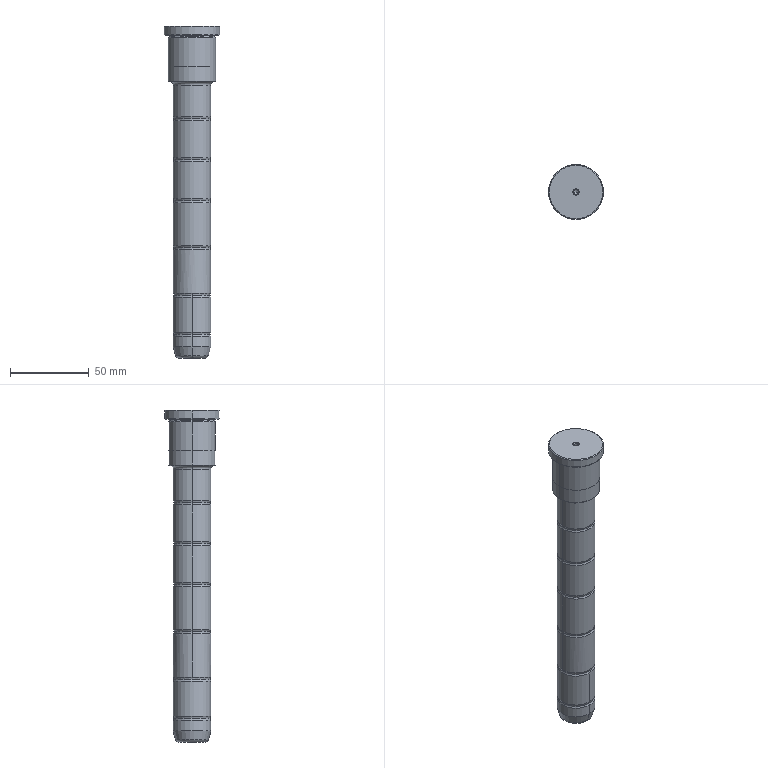Part | STEP file | Coluna inferior | 1 solid | 79 faces | box 35 x 35 x 211 mm | volume 105088 mm3 | torus 32 | cylinder 24 | cone 18 | plane 5 | commonest cylinder face diameters 24 x14 3 x4 29.98 x2 30 x2 35 x2